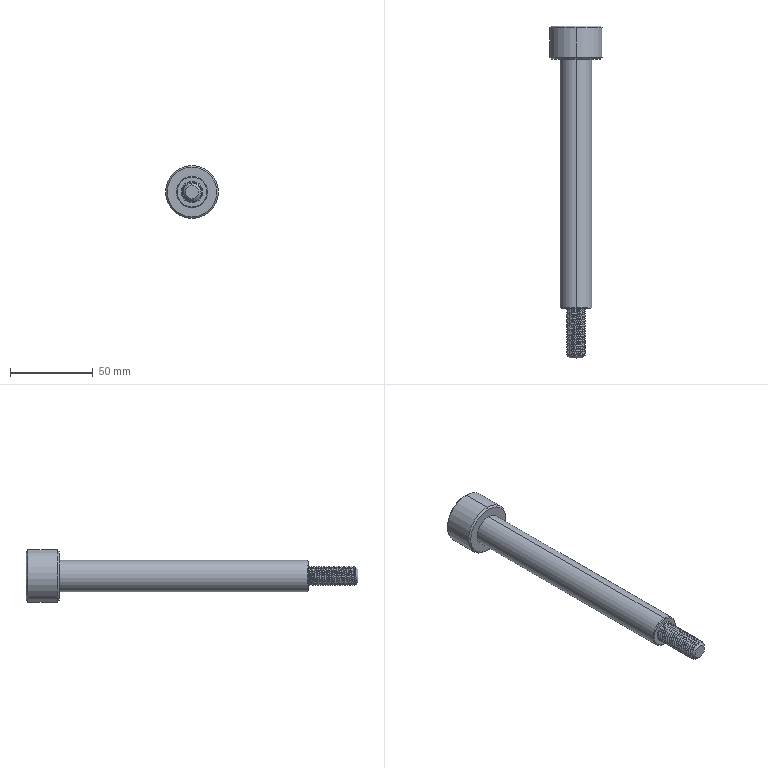Part | STEP file | Parafuso de retorno M12 - Torre - 1 cav | 1 solid | 74 faces | box 32 x 201 x 32 mm | volume 61230 mm3 | cylinder 42 | cone 12 | plane 11 | spline 7 | torus 2 | commonest cylinder face diameters 12 x38 19 x2 32 x2